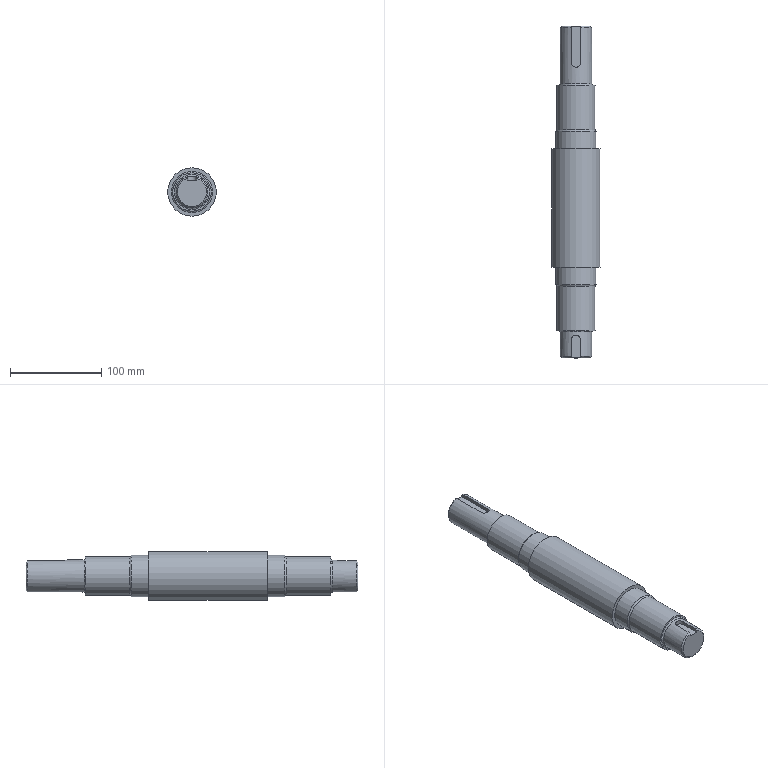Part | NX | features DATUM_CSYS 3, SKETCH 2, BLEND 1, CHAMFER 1, DATUM_PLANE 1, EXTRUDE 1, SWP104 1 | 1 solid | 27 faces | box 53 x 363 x 53 mm | volume 574308 mm3 | plane 12 | cylinder 9 | torus 4 | cone 2 | commonest cylinder face diameters 10 x2 35 x2 42 x2 45 x2 53 x1
STEP:
#1=CARTESIAN_POINT('',(-5.,0.,15.093));
#2=VERTEX_POINT('',#1);
#3=CARTESIAN_POINT('',(-5.,0.,13.));
#4=VERTEX_POINT('',#3);
#5=CARTESIAN_POINT('',(-5.,0.,17.5));
#6=DIRECTION('',(0.,0.,-1.));
#7=VECTOR('',#6,1000.);
#8=LINE('',#5,#7);
#9=EDGE_CURVE('',#2,#4,#8,.T.);
#10=ORIENTED_EDGE('',*,*,#9,.F.);
#11=CARTESIAN_POINT('',(5.,0.,15.093));
#12=VERTEX_POINT('',#11);
#13=CARTESIAN_POINT('',(0.,0.,0.));
#14=DIRECTION('',(0.,-1.,0.));
#15=DIRECTION('',(0.,0.,-1.));
#16=AXIS2_PLACEMENT_3D('',#13,#14,#15);
#17=CIRCLE('',#16,15.9);
#18=EDGE_CURVE('',#2,#12,#17,.T.);
#19=ORIENTED_EDGE('',*,*,#18,.T.);
#20=CARTESIAN_POINT('',(5.,0.,13.));
#21=VERTEX_POINT('',#20);
#22=CARTESIAN_POINT('',(5.,0.,17.5));
#23=DIRECTION('',(0.,0.,1.));
#24=VECTOR('',#23,1000.);
#25=LINE('',#22,#24);
#26=EDGE_CURVE('',#21,#12,#25,.T.);
#27=ORIENTED_EDGE('',*,*,#26,.F.);
#28=CARTESIAN_POINT('',(0.,0.,13.));
#29=DIRECTION('',(1.,0.,0.));
#30=VECTOR('',#29,1000.);
#31=LINE('',#28,#30);
#32=EDGE_CURVE('',#4,#21,#31,.T.);
#33=ORIENTED_EDGE('',*,*,#32,.F.);
#34=EDGE_LOOP('',(#10,#19,#27,#33));
#35=FACE_BOUND('',#34,.T.);
#36=CARTESIAN_POINT('',(0.,0.,17.5));
#37=DIRECTION('',(0.,-1.,0.));
#38=DIRECTION('',(0.,0.,-1.));
#39=AXIS2_PLACEMENT_3D('',#36,#37,#38);
#40=PLANE('',#39);
#41=ADVANCED_FACE('',(#35),#40,.T.);
#42=CARTESIAN_POINT('',(-5.,363.,13.));
#43=VERTEX_POINT('',#42);
#44=CARTESIAN_POINT('',(-5.,363.,15.093));
#45=VERTEX_POINT('',#44);
#46=CARTESIAN_POINT('',(-5.,363.,0.));
#47=DIRECTION('',(0.,0.,1.));
#48=VECTOR('',#47,1000.);
#49=LINE('',#46,#48);
#50=EDGE_CURVE('',#43,#45,#49,.T.);
#51=ORIENTED_EDGE('',*,*,#50,.F.);
#52=CARTESIAN_POINT('',(5.,363.,13.));
#53=VERTEX_POINT('',#52);
#54=CARTESIAN_POINT('',(0.,363.,13.));
#55=DIRECTION('',(-1.,0.,0.));
#56=VECTOR('',#55,1000.);
#57=LINE('',#54,#56);
#58=EDGE_CURVE('',#53,#43,#57,.T.);
#59=ORIENTED_EDGE('',*,*,#58,.F.);
#60=CARTESIAN_POINT('',(5.,363.,15.093));
#61=VERTEX_POINT('',#60);
#62=CARTESIAN_POINT('',(5.,363.,0.));
#63=DIRECTION('',(0.,0.,-1.));
#64=VECTOR('',#63,1000.);
#65=LINE('',#62,#64);
#66=EDGE_CURVE('',#61,#53,#65,.T.);
#67=ORIENTED_EDGE('',*,*,#66,.F.);
#68=CARTESIAN_POINT('',(0.,363.,0.));
#69=DIRECTION('',(0.,1.,0.));
#70=DIRECTION('',(0.,0.,1.));
#71=AXIS2_PLACEMENT_3D('',#68,#69,#70);
#72=CIRCLE('',#71,15.9);
#73=EDGE_CURVE('',#61,#45,#72,.T.);
#74=ORIENTED_EDGE('',*,*,#73,.T.);
#75=EDGE_LOOP('',(#51,#59,#67,#74));
#76=FACE_BOUND('',#75,.T.);
#77=CARTESIAN_POINT('',(0.,363.,0.));
#78=DIRECTION('',(0.,1.,0.));
#79=DIRECTION('',(0.,0.,1.));
#80=AXIS2_PLACEMENT_3D('',#77,#78,#79);
#81=PLANE('',#80);
#82=ADVANCED_FACE('',(#76),#81,.T.);
#83=CARTESIAN_POINT('',(-5.,361.4,16.771));
#84=VERTEX_POINT('',#83);
#85=CARTESIAN_POINT('',(-5.,323.,16.771));
#86=VERTEX_POINT('',#85);
#87=CARTESIAN_POINT('',(-5.,0.,16.771));
#88=DIRECTION('',(0.,1.,0.));
#89=VECTOR('',#88,1000.);
#90=LINE('',#87,#89);
#91=EDGE_CURVE('',#84,#86,#90,.F.);
#92=ORIENTED_EDGE('',*,*,#91,.F.);
#93=CARTESIAN_POINT('',(5.,361.4,16.771));
#94=VERTEX_POINT('',#93);
#95=CARTESIAN_POINT('',(0.,361.4,0.));
#96=DIRECTION('',(0.,1.,0.));
#97=DIRECTION('',(0.,0.,1.));
#98=AXIS2_PLACEMENT_3D('',#95,#96,#97);
#99=CIRCLE('',#98,17.5);
#100=EDGE_CURVE('',#84,#94,#99,.F.);
#101=ORIENTED_EDGE('',*,*,#100,.T.);
#102=CARTESIAN_POINT('',(5.,323.,16.771));
#103=VERTEX_POINT('',#102);
#104=CARTESIAN_POINT('',(5.,0.,16.771));
#105=DIRECTION('',(0.,1.,0.));
#106=VECTOR('',#105,1000.);
#107=LINE('',#104,#106);
#108=EDGE_CURVE('',#103,#94,#107,.T.);
#109=ORIENTED_EDGE('',*,*,#108,.F.);
#110=CARTESIAN_POINT('',(-5.,323.,16.771));
#111=CARTESIAN_POINT('',(-5.,321.671,16.771));
#112=CARTESIAN_POINT('',(-3.916,319.093,17.143));
#113=CARTESIAN_POINT('',(-0.007674,317.454,17.678));
#114=CARTESIAN_POINT('',(3.918,319.091,17.143));
#115=CARTESIAN_POINT('',(5.,321.671,16.771));
#116=CARTESIAN_POINT('',(5.,323.,16.771));
#117=B_SPLINE_CURVE_WITH_KNOTS('',3,(#110,#111,#112,#113,#114,#115,#116),.UNSPECIFIED.,.F.,.F.,(4,1,1,1,4),(0.,0.003927,0.007855,0.01178,0.01571),.UNSPECIFIED.);
#118=EDGE_CURVE('',#86,#103,#117,.T.);
#119=ORIENTED_EDGE('',*,*,#118,.F.);
#120=EDGE_LOOP('',(#92,#101,#109,#119));
#121=FACE_BOUND('',#120,.T.);
#122=CARTESIAN_POINT('',(0.,299.6,17.5));
#123=VERTEX_POINT('',#122);
#124=CARTESIAN_POINT('',(0.,299.6,0.));
#125=DIRECTION('',(0.,1.,0.));
#126=DIRECTION('',(0.,0.,1.));
#127=AXIS2_PLACEMENT_3D('',#124,#125,#126);
#128=CIRCLE('',#127,17.5);
#129=EDGE_CURVE('',#123,#123,#128,.T.);
#130=ORIENTED_EDGE('',*,*,#129,.T.);
#131=EDGE_LOOP('',(#130));
#132=FACE_BOUND('',#131,.T.);
#133=CARTESIAN_POINT('',(0.,0.,0.));
#134=DIRECTION('',(0.,1.,0.));
#135=DIRECTION('',(0.,0.,1.));
#136=AXIS2_PLACEMENT_3D('',#133,#134,#135);
#137=CYLINDRICAL_SURFACE('',#136,17.5);
#138=ADVANCED_FACE('',(#121,#132),#137,.T.);
#139=CARTESIAN_POINT('',(0.,298.,19.1));
#140=VERTEX_POINT('',#139);
#141=CARTESIAN_POINT('',(0.,298.,0.));
#142=DIRECTION('',(0.,1.,0.));
#143=DIRECTION('',(0.,0.,1.));
#144=AXIS2_PLACEMENT_3D('',#141,#142,#143);
#145=CIRCLE('',#144,19.1);
#146=EDGE_CURVE('',#140,#140,#145,.F.);
#147=ORIENTED_EDGE('',*,*,#146,.T.);
#148=EDGE_LOOP('',(#147));
#149=FACE_BOUND('',#148,.T.);
#150=CARTESIAN_POINT('',(0.,298.,21.));
#151=VERTEX_POINT('',#150);
#152=CARTESIAN_POINT('',(0.,298.,0.));
#153=DIRECTION('',(0.,1.,0.));
#154=DIRECTION('',(0.,0.,1.));
#155=AXIS2_PLACEMENT_3D('',#152,#153,#154);
#156=CIRCLE('',#155,21.);
#157=EDGE_CURVE('',#151,#151,#156,.T.);
#158=ORIENTED_EDGE('',*,*,#157,.T.);
#159=EDGE_LOOP('',(#158));
#160=FACE_BOUND('',#159,.T.);
#161=CARTESIAN_POINT('',(0.,298.,17.5));
#162=DIRECTION('',(0.,1.,0.));
#163=DIRECTION('',(0.,0.,1.));
#164=AXIS2_PLACEMENT_3D('',#161,#162,#163);
#165=PLANE('',#164);
#166=ADVANCED_FACE('',(#149,#160),#165,.T.);
#167=CARTESIAN_POINT('',(0.,249.597,-21.));
#168=VERTEX_POINT('',#167);
#169=CARTESIAN_POINT('',(0.,249.597,0.));
#170=DIRECTION('',(0.,-1.,0.));
#171=DIRECTION('',(0.,0.,-1.));
#172=AXIS2_PLACEMENT_3D('',#169,#170,#171);
#173=CIRCLE('',#172,21.);
#174=EDGE_CURVE('',#168,#168,#173,.F.);
#175=ORIENTED_EDGE('',*,*,#174,.T.);
#176=EDGE_LOOP('',(#175));
#177=FACE_BOUND('',#176,.T.);
#178=ORIENTED_EDGE('',*,*,#157,.F.);
#179=EDGE_LOOP('',(#178));
#180=FACE_BOUND('',#179,.T.);
#181=CARTESIAN_POINT('',(0.,0.,0.));
#182=DIRECTION('',(0.,1.,0.));
#183=DIRECTION('',(0.,0.,1.));
#184=AXIS2_PLACEMENT_3D('',#181,#182,#183);
#185=CYLINDRICAL_SURFACE('',#184,21.);
#186=ADVANCED_FACE('',(#177,#180),#185,.T.);
#187=CARTESIAN_POINT('',(0.,229.,22.5));
#188=VERTEX_POINT('',#187);
#189=CARTESIAN_POINT('',(0.,229.,0.));
#190=DIRECTION('',(0.,1.,0.));
#191=DIRECTION('',(0.,0.,1.));
#192=AXIS2_PLACEMENT_3D('',#189,#190,#191);
#193=CIRCLE('',#192,22.5);
#194=EDGE_CURVE('',#188,#188,#193,.T.);
#195=ORIENTED_EDGE('',*,*,#194,.T.);
#196=EDGE_LOOP('',(#195));
#197=FACE_BOUND('',#196,.T.);
#198=CARTESIAN_POINT('',(0.,248.,22.5));
#199=VERTEX_POINT('',#198);
#200=CARTESIAN_POINT('',(0.,248.,0.));
#201=DIRECTION('',(0.,1.,0.));
#202=DIRECTION('',(0.,0.,1.));
#203=AXIS2_PLACEMENT_3D('',#200,#201,#202);
#204=CIRCLE('',#203,22.5);
#205=EDGE_CURVE('',#199,#199,#204,.T.);
#206=ORIENTED_EDGE('',*,*,#205,.F.);
#207=EDGE_LOOP('',(#206));
#208=FACE_BOUND('',#207,.T.);
#209=CARTESIAN_POINT('',(0.,0.,0.));
#210=DIRECTION('',(0.,1.,0.));
#211=DIRECTION('',(0.,0.,1.));
#212=AXIS2_PLACEMENT_3D('',#209,#210,#211);
#213=CYLINDRICAL_SURFACE('',#212,22.5);
#214=ADVANCED_FACE('',(#197,#208),#213,.T.);
#215=CARTESIAN_POINT('',(0.,229.,26.5));
#216=VERTEX_POINT('',#215);
#217=CARTESIAN_POINT('',(0.,229.,0.));
#218=DIRECTION('',(0.,1.,0.));
#219=DIRECTION('',(0.,0.,1.));
#220=AXIS2_PLACEMENT_3D('',#217,#218,#219);
#221=CIRCLE('',#220,26.5);
#222=EDGE_CURVE('',#216,#216,#221,.T.);
#223=ORIENTED_EDGE('',*,*,#222,.T.);
#224=EDGE_LOOP('',(#223));
#225=FACE_BOUND('',#224,.T.);
#226=ORIENTED_EDGE('',*,*,#194,.F.);
#227=EDGE_LOOP('',(#226));
#228=FACE_BOUND('',#227,.T.);
#229=CARTESIAN_POINT('',(0.,229.,22.5));
#230=DIRECTION('',(0.,1.,0.));
#231=DIRECTION('',(0.,0.,1.));
#232=AXIS2_PLACEMENT_3D('',#229,#230,#231);
#233=PLANE('',#232);
#234=ADVANCED_FACE('',(#225,#228),#233,.T.);
#235=CARTESIAN_POINT('',(0.,99.,26.5));
#236=VERTEX_POINT('',#235);
#237=CARTESIAN_POINT('',(0.,99.,0.));
#238=DIRECTION('',(0.,1.,0.));
#239=DIRECTION('',(0.,0.,1.));
#240=AXIS2_PLACEMENT_3D('',#237,#238,#239);
#241=CIRCLE('',#240,26.5);
#242=EDGE_CURVE('',#236,#236,#241,.T.);
#243=ORIENTED_EDGE('',*,*,#242,.T.);
#244=EDGE_LOOP('',(#243));
#245=FACE_BOUND('',#244,.T.);
#246=ORIENTED_EDGE('',*,*,#222,.F.);
#247=EDGE_LOOP('',(#246));
#248=FACE_BOUND('',#247,.T.);
#249=CARTESIAN_POINT('',(0.,0.,0.));
#250=DIRECTION('',(0.,1.,0.));
#251=DIRECTION('',(0.,0.,1.));
#252=AXIS2_PLACEMENT_3D('',#249,#250,#251);
#253=CYLINDRICAL_SURFACE('',#252,26.5);
#254=ADVANCED_FACE('',(#245,#248),#253,.T.);
#255=CARTESIAN_POINT('',(0.,99.,22.5));
#256=VERTEX_POINT('',#255);
#257=CARTESIAN_POINT('',(0.,99.,0.));
#258=DIRECTION('',(0.,1.,0.));
#259=DIRECTION('',(0.,0.,1.));
#260=AXIS2_PLACEMENT_3D('',#257,#258,#259);
#261=CIRCLE('',#260,22.5);
#262=EDGE_CURVE('',#256,#256,#261,.T.);
#263=ORIENTED_EDGE('',*,*,#262,.T.);
#264=EDGE_LOOP('',(#263));
#265=FACE_BOUND('',#264,.T.);
#266=ORIENTED_EDGE('',*,*,#242,.F.);
#267=EDGE_LOOP('',(#266));
#268=FACE_BOUND('',#267,.T.);
#269=CARTESIAN_POINT('',(0.,99.,26.5));
#270=DIRECTION('',(0.,-1.,0.));
#271=DIRECTION('',(0.,0.,-1.));
#272=AXIS2_PLACEMENT_3D('',#269,#270,#271);
#273=PLANE('',#272);
#274=ADVANCED_FACE('',(#265,#268),#273,.T.);
#275=CARTESIAN_POINT('',(0.,80.,22.5));
#276=VERTEX_POINT('',#275);
#277=CARTESIAN_POINT('',(0.,80.,0.));
#278=DIRECTION('',(0.,1.,0.));
#279=DIRECTION('',(0.,0.,1.));
#280=AXIS2_PLACEMENT_3D('',#277,#278,#279);
#281=CIRCLE('',#280,22.5);
#282=EDGE_CURVE('',#276,#276,#281,.T.);
#283=ORIENTED_EDGE('',*,*,#282,.T.);
#284=EDGE_LOOP('',(#283));
#285=FACE_BOUND('',#284,.T.);
#286=ORIENTED_EDGE('',*,*,#262,.F.);
#287=EDGE_LOOP('',(#286));
#288=FACE_BOUND('',#287,.T.);
#289=CARTESIAN_POINT('',(0.,0.,0.));
#290=DIRECTION('',(0.,1.,0.));
#291=DIRECTION('',(0.,0.,1.));
#292=AXIS2_PLACEMENT_3D('',#289,#290,#291);
#293=CYLINDRICAL_SURFACE('',#292,22.5);
#294=ADVANCED_FACE('',(#285,#288),#293,.T.);
#295=CARTESIAN_POINT('',(0.,78.403,21.));
#296=VERTEX_POINT('',#295);
#297=CARTESIAN_POINT('',(0.,78.403,0.));
#298=DIRECTION('',(0.,1.,0.));
#299=DIRECTION('',(0.,0.,1.));
#300=AXIS2_PLACEMENT_3D('',#297,#298,#299);
#301=CIRCLE('',#300,21.);
#302=EDGE_CURVE('',#296,#296,#301,.F.);
#303=ORIENTED_EDGE('',*,*,#302,.T.);
#304=EDGE_LOOP('',(#303));
#305=FACE_BOUND('',#304,.T.);
#306=CARTESIAN_POINT('',(0.,30.,21.));
#307=VERTEX_POINT('',#306);
#308=CARTESIAN_POINT('',(0.,30.,0.));
#309=DIRECTION('',(0.,1.,0.));
#310=DIRECTION('',(0.,0.,1.));
#311=AXIS2_PLACEMENT_3D('',#308,#309,#310);
#312=CIRCLE('',#311,21.);
#313=EDGE_CURVE('',#307,#307,#312,.T.);
#314=ORIENTED_EDGE('',*,*,#313,.T.);
#315=EDGE_LOOP('',(#314));
#316=FACE_BOUND('',#315,.T.);
#317=CARTESIAN_POINT('',(0.,0.,0.));
#318=DIRECTION('',(0.,1.,0.));
#319=DIRECTION('',(0.,0.,1.));
#320=AXIS2_PLACEMENT_3D('',#317,#318,#319);
#321=CYLINDRICAL_SURFACE('',#320,21.);
#322=ADVANCED_FACE('',(#305,#316),#321,.T.);
#323=CARTESIAN_POINT('',(0.,30.,-19.1));
#324=VERTEX_POINT('',#323);
#325=CARTESIAN_POINT('',(0.,30.,0.));
#326=DIRECTION('',(0.,-1.,0.));
#327=DIRECTION('',(0.,0.,-1.));
#328=AXIS2_PLACEMENT_3D('',#325,#326,#327);
#329=CIRCLE('',#328,19.1);
#330=EDGE_CURVE('',#324,#324,#329,.F.);
#331=ORIENTED_EDGE('',*,*,#330,.T.);
#332=EDGE_LOOP('',(#331));
#333=FACE_BOUND('',#332,.T.);
#334=ORIENTED_EDGE('',*,*,#313,.F.);
#335=EDGE_LOOP('',(#334));
#336=FACE_BOUND('',#335,.T.);
#337=CARTESIAN_POINT('',(0.,30.,21.));
#338=DIRECTION('',(0.,-1.,0.));
#339=DIRECTION('',(0.,0.,-1.));
#340=AXIS2_PLACEMENT_3D('',#337,#338,#339);
#341=PLANE('',#340);
#342=ADVANCED_FACE('',(#333,#336),#341,.T.);
#343=CARTESIAN_POINT('',(-5.,20.,16.771));
#344=VERTEX_POINT('',#343);
#345=CARTESIAN_POINT('',(-5.,1.6,16.771));
#346=VERTEX_POINT('',#345);
#347=CARTESIAN_POINT('',(-5.,0.,16.771));
#348=DIRECTION('',(0.,1.,0.));
#349=VECTOR('',#348,1000.);
#350=LINE('',#347,#349);
#351=EDGE_CURVE('',#344,#346,#350,.F.);
#352=ORIENTED_EDGE('',*,*,#351,.F.);
#353=CARTESIAN_POINT('',(5.,20.,16.771));
#354=VERTEX_POINT('',#353);
#355=CARTESIAN_POINT('',(5.,20.,16.771));
#356=CARTESIAN_POINT('',(5.,21.329,16.771));
#357=CARTESIAN_POINT('',(3.916,23.907,17.143));
#358=CARTESIAN_POINT('',(0.007674,25.546,17.678));
#359=CARTESIAN_POINT('',(-3.918,23.909,17.143));
#360=CARTESIAN_POINT('',(-5.,21.329,16.771));
#361=CARTESIAN_POINT('',(-5.,20.,16.771));
#362=B_SPLINE_CURVE_WITH_KNOTS('',3,(#355,#356,#357,#358,#359,#360,#361),.UNSPECIFIED.,.F.,.F.,(4,1,1,1,4),(0.,0.003927,0.007855,0.01178,0.01571),.UNSPECIFIED.);
#363=EDGE_CURVE('',#354,#344,#362,.T.);
#364=ORIENTED_EDGE('',*,*,#363,.F.);
#365=CARTESIAN_POINT('',(5.,1.6,16.771));
#366=VERTEX_POINT('',#365);
#367=CARTESIAN_POINT('',(5.,0.,16.771));
#368=DIRECTION('',(0.,1.,0.));
#369=VECTOR('',#368,1000.);
#370=LINE('',#367,#369);
#371=EDGE_CURVE('',#366,#354,#370,.T.);
#372=ORIENTED_EDGE('',*,*,#371,.F.);
#373=CARTESIAN_POINT('',(0.,1.6,0.));
#374=DIRECTION('',(0.,-1.,0.));
#375=DIRECTION('',(0.,0.,-1.));
#376=AXIS2_PLACEMENT_3D('',#373,#374,#375);
#377=CIRCLE('',#376,17.5);
#378=EDGE_CURVE('',#366,#346,#377,.F.);
#379=ORIENTED_EDGE('',*,*,#378,.T.);
#380=EDGE_LOOP('',(#352,#364,#372,#379));
#381=FACE_BOUND('',#380,.T.);
#382=CARTESIAN_POINT('',(0.,28.4,-17.5));
#383=VERTEX_POINT('',#382);
#384=CARTESIAN_POINT('',(0.,28.4,0.));
#385=DIRECTION('',(0.,-1.,0.));
#386=DIRECTION('',(0.,0.,-1.));
#387=AXIS2_PLACEMENT_3D('',#384,#385,#386);
#388=CIRCLE('',#387,17.5);
#389=EDGE_CURVE('',#383,#383,#388,.T.);
#390=ORIENTED_EDGE('',*,*,#389,.T.);
#391=EDGE_LOOP('',(#390));
#392=FACE_BOUND('',#391,.T.);
#393=CARTESIAN_POINT('',(0.,0.,0.));
#394=DIRECTION('',(0.,1.,0.));
#395=DIRECTION('',(0.,0.,1.));
#396=AXIS2_PLACEMENT_3D('',#393,#394,#395);
#397=CYLINDRICAL_SURFACE('',#396,17.5);
#398=ADVANCED_FACE('',(#381,#392),#397,.T.);
#399=CARTESIAN_POINT('',(-5.,1.6,16.771));
#400=CARTESIAN_POINT('',(-5.,1.065,16.213));
#401=CARTESIAN_POINT('',(-5.,0.5319,15.654));
#402=CARTESIAN_POINT('',(-5.,0.,15.093));
#403=B_SPLINE_CURVE_WITH_KNOTS('',3,(#399,#400,#401,#402),.UNSPECIFIED.,.F.,.F.,(4,4),(0.007353,0.009671),.UNSPECIFIED.);
#404=EDGE_CURVE('',#346,#2,#403,.T.);
#405=ORIENTED_EDGE('',*,*,#404,.F.);
#406=ORIENTED_EDGE('',*,*,#378,.F.);
#407=CARTESIAN_POINT('',(5.,0.,15.093));
#408=CARTESIAN_POINT('',(5.,0.5319,15.654));
#409=CARTESIAN_POINT('',(5.,1.065,16.213));
#410=CARTESIAN_POINT('',(5.,1.6,16.771));
#411=B_SPLINE_CURVE_WITH_KNOTS('',3,(#407,#408,#409,#410),.UNSPECIFIED.,.F.,.F.,(4,4),(0.009162,0.01148),.UNSPECIFIED.);
#412=EDGE_CURVE('',#12,#366,#411,.T.);
#413=ORIENTED_EDGE('',*,*,#412,.F.);
#414=ORIENTED_EDGE('',*,*,#18,.F.);
#415=EDGE_LOOP('',(#405,#406,#413,#414));
#416=FACE_BOUND('',#415,.T.);
#417=CARTESIAN_POINT('',(0.,1.6,0.));
#418=DIRECTION('',(0.,1.,0.));
#419=DIRECTION('',(0.,0.,1.));
#420=AXIS2_PLACEMENT_3D('',#417,#418,#419);
#421=CONICAL_SURFACE('',#420,17.5,0.7854);
#422=ADVANCED_FACE('',(#416),#421,.T.);
#423=CARTESIAN_POINT('',(-5.,363.,15.093));
#424=CARTESIAN_POINT('',(-5.,362.468,15.654));
#425=CARTESIAN_POINT('',(-5.,361.935,16.213));
#426=CARTESIAN_POINT('',(-5.,361.4,16.771));
#427=B_SPLINE_CURVE_WITH_KNOTS('',3,(#423,#424,#425,#426),.UNSPECIFIED.,.F.,.F.,(4,4),(0.009162,0.01148),.UNSPECIFIED.);
#428=EDGE_CURVE('',#45,#84,#427,.T.);
#429=ORIENTED_EDGE('',*,*,#428,.F.);
#430=ORIENTED_EDGE('',*,*,#73,.F.);
#431=CARTESIAN_POINT('',(5.,361.4,16.771));
#432=CARTESIAN_POINT('',(5.,361.935,16.213));
#433=CARTESIAN_POINT('',(5.,362.468,15.654));
#434=CARTESIAN_POINT('',(5.,363.,15.093));
#435=B_SPLINE_CURVE_WITH_KNOTS('',3,(#431,#432,#433,#434),.UNSPECIFIED.,.F.,.F.,(4,4),(0.007353,0.009671),.UNSPECIFIED.);
#436=EDGE_CURVE('',#94,#61,#435,.T.);
#437=ORIENTED_EDGE('',*,*,#436,.F.);
#438=ORIENTED_EDGE('',*,*,#100,.F.);
#439=EDGE_LOOP('',(#429,#430,#437,#438));
#440=FACE_BOUND('',#439,.T.);
#441=CARTESIAN_POINT('',(0.,363.,0.));
#442=DIRECTION('',(0.,-1.,0.));
#443=DIRECTION('',(0.,0.,-1.));
#444=AXIS2_PLACEMENT_3D('',#441,#442,#443);
#445=CONICAL_SURFACE('',#444,15.9,0.7854);
#446=ADVANCED_FACE('',(#440),#445,.T.);
#447=ORIENTED_EDGE('',*,*,#302,.F.);
#448=EDGE_LOOP('',(#447));
#449=FACE_BOUND('',#448,.T.);
#450=ORIENTED_EDGE('',*,*,#282,.F.);
#451=EDGE_LOOP('',(#450));
#452=FACE_BOUND('',#451,.T.);
#453=CARTESIAN_POINT('',(0.,78.403,0.));
#454=DIRECTION('',(0.,1.,0.));
#455=DIRECTION('',(0.,0.,1.));
#456=AXIS2_PLACEMENT_3D('',#453,#454,#455);
#457=TOROIDAL_SURFACE('',#456,22.6,1.6);
#458=ADVANCED_FACE('',(#449,#452),#457,.F.);
#459=ORIENTED_EDGE('',*,*,#205,.T.);
#460=EDGE_LOOP('',(#459));
#461=FACE_BOUND('',#460,.T.);
#462=ORIENTED_EDGE('',*,*,#174,.F.);
#463=EDGE_LOOP('',(#462));
#464=FACE_BOUND('',#463,.T.);
#465=CARTESIAN_POINT('',(0.,249.597,0.));
#466=DIRECTION('',(0.,-1.,0.));
#467=DIRECTION('',(0.,0.,-1.));
#468=AXIS2_PLACEMENT_3D('',#465,#466,#467);
#469=TOROIDAL_SURFACE('',#468,22.6,1.6);
#470=ADVANCED_FACE('',(#461,#464),#469,.F.);
#471=ORIENTED_EDGE('',*,*,#389,.F.);
#472=EDGE_LOOP('',(#471));
#473=FACE_BOUND('',#472,.T.);
#474=ORIENTED_EDGE('',*,*,#330,.F.);
#475=EDGE_LOOP('',(#474));
#476=FACE_BOUND('',#475,.T.);
#477=CARTESIAN_POINT('',(0.,28.4,0.));
#478=DIRECTION('',(0.,-1.,0.));
#479=DIRECTION('',(0.,0.,-1.));
#480=AXIS2_PLACEMENT_3D('',#477,#478,#479);
#481=TOROIDAL_SURFACE('',#480,19.1,1.6);
#482=ADVANCED_FACE('',(#473,#476),#481,.F.);
#483=ORIENTED_EDGE('',*,*,#146,.F.);
#484=EDGE_LOOP('',(#483));
#485=FACE_BOUND('',#484,.T.);
#486=ORIENTED_EDGE('',*,*,#129,.F.);
#487=EDGE_LOOP('',(#486));
#488=FACE_BOUND('',#487,.T.);
#489=CARTESIAN_POINT('',(0.,299.6,0.));
#490=DIRECTION('',(0.,1.,0.));
#491=DIRECTION('',(0.,0.,1.));
#492=AXIS2_PLACEMENT_3D('',#489,#490,#491);
#493=TOROIDAL_SURFACE('',#492,19.1,1.6);
#494=ADVANCED_FACE('',(#485,#488),#493,.F.);
#495=ORIENTED_EDGE('',*,*,#9,.T.);
#496=CARTESIAN_POINT('',(-5.,20.,13.));
#497=VERTEX_POINT('',#496);
#498=CARTESIAN_POINT('',(-5.,-30.,13.));
#499=DIRECTION('',(0.,1.,0.));
#500=VECTOR('',#499,1000.);
#501=LINE('',#498,#500);
#502=EDGE_CURVE('',#497,#4,#501,.F.);
#503=ORIENTED_EDGE('',*,*,#502,.F.);
#504=CARTESIAN_POINT('',(-5.,20.,73.));
#505=DIRECTION('',(0.,0.,-1.));
#506=VECTOR('',#505,1000.);
#507=LINE('',#504,#506);
#508=EDGE_CURVE('',#497,#344,#507,.F.);
#509=ORIENTED_EDGE('',*,*,#508,.T.);
#510=ORIENTED_EDGE('',*,*,#351,.T.);
#511=ORIENTED_EDGE('',*,*,#404,.T.);
#512=EDGE_LOOP('',(#495,#503,#509,#510,#511));
#513=FACE_BOUND('',#512,.T.);
#514=CARTESIAN_POINT('',(-5.,-30.,73.));
#515=DIRECTION('',(-1.,0.,0.));
#516=DIRECTION('',(0.,-1.,0.));
#517=AXIS2_PLACEMENT_3D('',#514,#515,#516);
#518=PLANE('',#517);
#519=ADVANCED_FACE('',(#513),#518,.F.);
#520=ORIENTED_EDGE('',*,*,#363,.T.);
#521=ORIENTED_EDGE('',*,*,#508,.F.);
#522=CARTESIAN_POINT('',(5.,20.,13.));
#523=VERTEX_POINT('',#522);
#524=CARTESIAN_POINT('',(0.,20.,13.));
#525=DIRECTION('',(0.,0.,-1.));
#526=DIRECTION('',(1.,0.,0.));
#527=AXIS2_PLACEMENT_3D('',#524,#525,#526);
#528=CIRCLE('',#527,5.);
#529=EDGE_CURVE('',#523,#497,#528,.F.);
#530=ORIENTED_EDGE('',*,*,#529,.F.);
#531=CARTESIAN_POINT('',(5.,20.,73.));
#532=DIRECTION('',(0.,0.,-1.));
#533=VECTOR('',#532,1000.);
#534=LINE('',#531,#533);
#535=EDGE_CURVE('',#523,#354,#534,.F.);
#536=ORIENTED_EDGE('',*,*,#535,.T.);
#537=EDGE_LOOP('',(#520,#521,#530,#536));
#538=FACE_BOUND('',#537,.T.);
#539=CARTESIAN_POINT('',(0.,20.,73.));
#540=DIRECTION('',(0.,0.,-1.));
#541=DIRECTION('',(-1.,0.,0.));
#542=AXIS2_PLACEMENT_3D('',#539,#540,#541);
#543=CYLINDRICAL_SURFACE('',#542,5.);
#544=ADVANCED_FACE('',(#538),#543,.F.);
#545=ORIENTED_EDGE('',*,*,#26,.T.);
#546=ORIENTED_EDGE('',*,*,#412,.T.);
#547=ORIENTED_EDGE('',*,*,#371,.T.);
#548=ORIENTED_EDGE('',*,*,#535,.F.);
#549=CARTESIAN_POINT('',(5.,20.,13.));
#550=DIRECTION('',(0.,-1.,0.));
#551=VECTOR('',#550,1000.);
#552=LINE('',#549,#551);
#553=EDGE_CURVE('',#21,#523,#552,.F.);
#554=ORIENTED_EDGE('',*,*,#553,.F.);
#555=EDGE_LOOP('',(#545,#546,#547,#548,#554));
#556=FACE_BOUND('',#555,.T.);
#557=CARTESIAN_POINT('',(5.,20.,73.));
#558=DIRECTION('',(1.,0.,0.));
#559=DIRECTION('',(0.,1.,0.));
#560=AXIS2_PLACEMENT_3D('',#557,#558,#559);
#561=PLANE('',#560);
#562=ADVANCED_FACE('',(#556),#561,.F.);
#563=ORIENTED_EDGE('',*,*,#32,.T.);
#564=ORIENTED_EDGE('',*,*,#553,.T.);
#565=ORIENTED_EDGE('',*,*,#529,.T.);
#566=ORIENTED_EDGE('',*,*,#502,.T.);
#567=EDGE_LOOP('',(#563,#564,#565,#566));
#568=FACE_BOUND('',#567,.T.);
#569=CARTESIAN_POINT('',(0.,20.,13.));
#570=DIRECTION('',(0.,0.,-1.));
#571=DIRECTION('',(-1.,0.,0.));
#572=AXIS2_PLACEMENT_3D('',#569,#570,#571);
#573=PLANE('',#572);
#574=ADVANCED_FACE('',(#568),#573,.F.);
#575=ORIENTED_EDGE('',*,*,#50,.T.);
#576=ORIENTED_EDGE('',*,*,#428,.T.);
#577=ORIENTED_EDGE('',*,*,#91,.T.);
#578=CARTESIAN_POINT('',(-5.,323.,13.));
#579=VERTEX_POINT('',#578);
#580=CARTESIAN_POINT('',(-5.,323.,73.));
#581=DIRECTION('',(0.,0.,-1.));
#582=VECTOR('',#581,1000.);
#583=LINE('',#580,#582);
#584=EDGE_CURVE('',#579,#86,#583,.F.);
#585=ORIENTED_EDGE('',*,*,#584,.F.);
#586=CARTESIAN_POINT('',(-5.,323.,13.));
#587=DIRECTION('',(0.,1.,0.));
#588=VECTOR('',#587,1000.);
#589=LINE('',#586,#588);
#590=EDGE_CURVE('',#43,#579,#589,.F.);
#591=ORIENTED_EDGE('',*,*,#590,.F.);
#592=EDGE_LOOP('',(#575,#576,#577,#585,#591));
#593=FACE_BOUND('',#592,.T.);
#594=CARTESIAN_POINT('',(-5.,323.,73.));
#595=DIRECTION('',(-1.,0.,0.));
#596=DIRECTION('',(0.,-1.,0.));
#597=AXIS2_PLACEMENT_3D('',#594,#595,#596);
#598=PLANE('',#597);
#599=ADVANCED_FACE('',(#593),#598,.F.);
#600=ORIENTED_EDGE('',*,*,#66,.T.);
#601=CARTESIAN_POINT('',(5.,323.,13.));
#602=VERTEX_POINT('',#601);
#603=CARTESIAN_POINT('',(5.,383.,13.));
#604=DIRECTION('',(0.,-1.,0.));
#605=VECTOR('',#604,1000.);
#606=LINE('',#603,#605);
#607=EDGE_CURVE('',#602,#53,#606,.F.);
#608=ORIENTED_EDGE('',*,*,#607,.F.);
#609=CARTESIAN_POINT('',(5.,323.,73.));
#610=DIRECTION('',(0.,0.,-1.));
#611=VECTOR('',#610,1000.);
#612=LINE('',#609,#611);
#613=EDGE_CURVE('',#602,#103,#612,.F.);
#614=ORIENTED_EDGE('',*,*,#613,.T.);
#615=ORIENTED_EDGE('',*,*,#108,.T.);
#616=ORIENTED_EDGE('',*,*,#436,.T.);
#617=EDGE_LOOP('',(#600,#608,#614,#615,#616));
#618=FACE_BOUND('',#617,.T.);
#619=CARTESIAN_POINT('',(5.,383.,73.));
#620=DIRECTION('',(1.,0.,0.));
#621=DIRECTION('',(0.,1.,0.));
#622=AXIS2_PLACEMENT_3D('',#619,#620,#621);
#623=PLANE('',#622);
#624=ADVANCED_FACE('',(#618),#623,.F.);
#625=ORIENTED_EDGE('',*,*,#118,.T.);
#626=ORIENTED_EDGE('',*,*,#613,.F.);
#627=CARTESIAN_POINT('',(0.,323.,13.));
#628=DIRECTION('',(0.,0.,-1.));
#629=DIRECTION('',(1.,0.,0.));
#630=AXIS2_PLACEMENT_3D('',#627,#628,#629);
#631=CIRCLE('',#630,5.);
#632=EDGE_CURVE('',#579,#602,#631,.F.);
#633=ORIENTED_EDGE('',*,*,#632,.F.);
#634=ORIENTED_EDGE('',*,*,#584,.T.);
#635=EDGE_LOOP('',(#625,#626,#633,#634));
#636=FACE_BOUND('',#635,.T.);
#637=CARTESIAN_POINT('',(0.,323.,73.));
#638=DIRECTION('',(0.,0.,-1.));
#639=DIRECTION('',(-1.,0.,0.));
#640=AXIS2_PLACEMENT_3D('',#637,#638,#639);
#641=CYLINDRICAL_SURFACE('',#640,5.);
#642=ADVANCED_FACE('',(#636),#641,.F.);
#643=ORIENTED_EDGE('',*,*,#58,.T.);
#644=ORIENTED_EDGE('',*,*,#590,.T.);
#645=ORIENTED_EDGE('',*,*,#632,.T.);
#646=ORIENTED_EDGE('',*,*,#607,.T.);
#647=EDGE_LOOP('',(#643,#644,#645,#646));
#648=FACE_BOUND('',#647,.T.);
#649=CARTESIAN_POINT('',(0.,323.,13.));
#650=DIRECTION('',(0.,0.,-1.));
#651=DIRECTION('',(-1.,0.,0.));
#652=AXIS2_PLACEMENT_3D('',#649,#650,#651);
#653=PLANE('',#652);
#654=ADVANCED_FACE('',(#648),#653,.F.);
#655=CLOSED_SHELL('',(#41,#82,#138,#166,#186,#214,#234,#254,#274,#294,#322,#342,#398,#422,#446,#458,#470,#482,#494,#519,#544,#562,#574,#599,#624,#642,#654));
#656=MANIFOLD_SOLID_BREP('',#655);
#657=(LENGTH_UNIT()NAMED_UNIT(*)SI_UNIT(.MILLI.,.METRE.));
#658=UNCERTAINTY_MEASURE_WITH_UNIT(LENGTH_MEASURE(0.0508),#657,'','');
#659=(NAMED_UNIT(*)PLANE_ANGLE_UNIT()SI_UNIT($,.RADIAN.));
#660=(NAMED_UNIT(*)SI_UNIT($,.STERADIAN.)SOLID_ANGLE_UNIT());
#661=(GEOMETRIC_REPRESENTATION_CONTEXT(3)GLOBAL_UNCERTAINTY_ASSIGNED_CONTEXT((#658))GLOBAL_UNIT_ASSIGNED_CONTEXT((#657,#659,#660))REPRESENTATION_CONTEXT('',''));
#662=ADVANCED_BREP_SHAPE_REPRESENTATION('',(#656),#661);